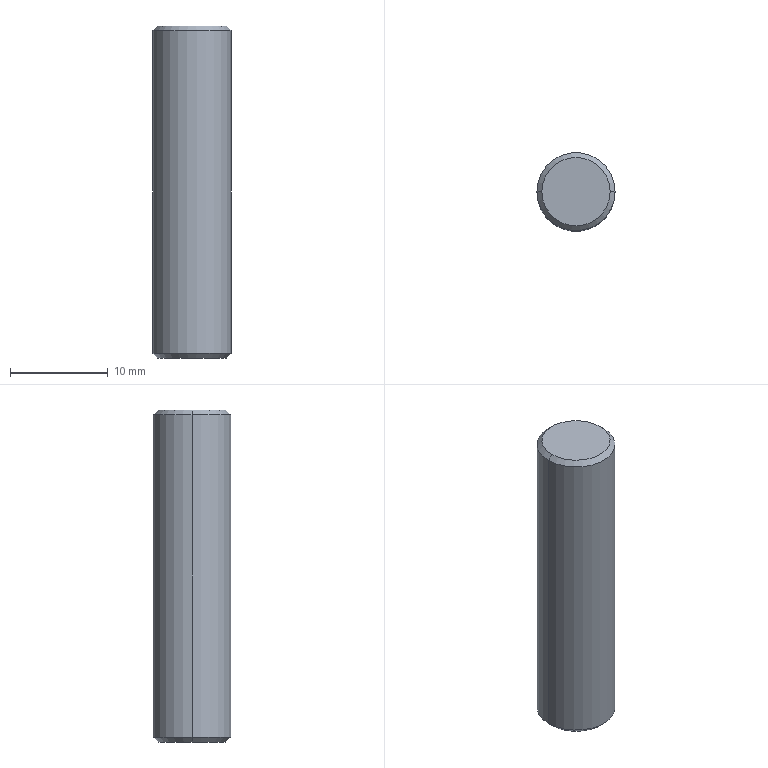Part | SolidWorks | features Chamfer 1, Extrusion 1 | 1 solid | 8 faces | box 8 x 8 x 34 mm | volume 1703 mm3 | cone 4 | cylinder 2 | plane 2 | commonest cylinder face diameters 8 x2
STEP:
#1=CARTESIAN_POINT('',(3.5,0.,17.));
#2=VERTEX_POINT('',#1);
#3=CARTESIAN_POINT('',(-3.5,0.,17.));
#4=VERTEX_POINT('',#3);
#5=CARTESIAN_POINT('',(0.,0.,17.));
#6=DIRECTION('',(0.,0.,1.));
#7=DIRECTION('',(1.,0.,0.));
#8=AXIS2_PLACEMENT_3D('',#5,#6,#7);
#9=CIRCLE('',#8,3.5);
#10=EDGE_CURVE('',#2,#4,#9,.T.);
#11=ORIENTED_EDGE('',*,*,#10,.F.);
#12=CARTESIAN_POINT('',(4.,0.,16.5));
#13=VERTEX_POINT('',#12);
#14=CARTESIAN_POINT('',(3.5,0.,17.));
#15=DIRECTION('',(0.7071,0.,-0.7071));
#16=VECTOR('',#15,1000.);
#17=LINE('',#14,#16);
#18=EDGE_CURVE('',#2,#13,#17,.T.);
#19=ORIENTED_EDGE('',*,*,#18,.T.);
#20=CARTESIAN_POINT('',(-4.,0.,16.5));
#21=VERTEX_POINT('',#20);
#22=CARTESIAN_POINT('',(0.,0.,16.5));
#23=DIRECTION('',(0.,0.,-1.));
#24=DIRECTION('',(1.,0.,0.));
#25=AXIS2_PLACEMENT_3D('',#22,#23,#24);
#26=CIRCLE('',#25,4.);
#27=EDGE_CURVE('',#21,#13,#26,.T.);
#28=ORIENTED_EDGE('',*,*,#27,.F.);
#29=CARTESIAN_POINT('',(-3.5,0.,17.));
#30=DIRECTION('',(-0.7071,0.,-0.7071));
#31=VECTOR('',#30,1000.);
#32=LINE('',#29,#31);
#33=EDGE_CURVE('',#4,#21,#32,.T.);
#34=ORIENTED_EDGE('',*,*,#33,.F.);
#35=EDGE_LOOP('',(#11,#19,#28,#34));
#36=FACE_OUTER_BOUND('',#35,.T.);
#37=CARTESIAN_POINT('',(0.,0.,17.));
#38=DIRECTION('',(0.,0.,-1.));
#39=DIRECTION('',(-1.,0.,0.));
#40=AXIS2_PLACEMENT_3D('',#37,#38,#39);
#41=CONICAL_SURFACE('',#40,3.5,0.7854);
#42=ADVANCED_FACE('',(#36),#41,.T.);
#43=CARTESIAN_POINT('',(-3.5,0.,-17.));
#44=VERTEX_POINT('',#43);
#45=CARTESIAN_POINT('',(3.5,0.,-17.));
#46=VERTEX_POINT('',#45);
#47=CARTESIAN_POINT('',(0.,0.,-17.));
#48=DIRECTION('',(0.,0.,-1.));
#49=DIRECTION('',(1.,0.,0.));
#50=AXIS2_PLACEMENT_3D('',#47,#48,#49);
#51=CIRCLE('',#50,3.5);
#52=EDGE_CURVE('',#44,#46,#51,.T.);
#53=ORIENTED_EDGE('',*,*,#52,.F.);
#54=CARTESIAN_POINT('',(-4.,0.,-16.5));
#55=VERTEX_POINT('',#54);
#56=CARTESIAN_POINT('',(-4.,0.,-16.5));
#57=DIRECTION('',(-0.7071,0.,0.7071));
#58=VECTOR('',#57,1000.);
#59=LINE('',#56,#58);
#60=EDGE_CURVE('',#44,#55,#59,.T.);
#61=ORIENTED_EDGE('',*,*,#60,.T.);
#62=CARTESIAN_POINT('',(4.,0.,-16.5));
#63=VERTEX_POINT('',#62);
#64=CARTESIAN_POINT('',(0.,0.,-16.5));
#65=DIRECTION('',(0.,0.,1.));
#66=DIRECTION('',(1.,0.,0.));
#67=AXIS2_PLACEMENT_3D('',#64,#65,#66);
#68=CIRCLE('',#67,4.);
#69=EDGE_CURVE('',#63,#55,#68,.T.);
#70=ORIENTED_EDGE('',*,*,#69,.F.);
#71=CARTESIAN_POINT('',(4.,0.,-16.5));
#72=DIRECTION('',(0.7071,0.,0.7071));
#73=VECTOR('',#72,1000.);
#74=LINE('',#71,#73);
#75=EDGE_CURVE('',#46,#63,#74,.T.);
#76=ORIENTED_EDGE('',*,*,#75,.F.);
#77=EDGE_LOOP('',(#53,#61,#70,#76));
#78=FACE_OUTER_BOUND('',#77,.T.);
#79=CARTESIAN_POINT('',(0.,0.,-16.5));
#80=DIRECTION('',(0.,0.,1.));
#81=DIRECTION('',(1.,0.,0.));
#82=AXIS2_PLACEMENT_3D('',#79,#80,#81);
#83=CONICAL_SURFACE('',#82,4.,0.7854);
#84=ADVANCED_FACE('',(#78),#83,.T.);
#85=ORIENTED_EDGE('',*,*,#27,.T.);
#86=CARTESIAN_POINT('',(4.,0.,17.));
#87=DIRECTION('',(0.,0.,-1.));
#88=VECTOR('',#87,1000.);
#89=LINE('',#86,#88);
#90=EDGE_CURVE('',#13,#63,#89,.T.);
#91=ORIENTED_EDGE('',*,*,#90,.T.);
#92=ORIENTED_EDGE('',*,*,#69,.T.);
#93=CARTESIAN_POINT('',(-4.,0.,17.));
#94=DIRECTION('',(0.,0.,-1.));
#95=VECTOR('',#94,1000.);
#96=LINE('',#93,#95);
#97=EDGE_CURVE('',#21,#55,#96,.T.);
#98=ORIENTED_EDGE('',*,*,#97,.F.);
#99=EDGE_LOOP('',(#85,#91,#92,#98));
#100=FACE_OUTER_BOUND('',#99,.T.);
#101=CARTESIAN_POINT('',(0.,0.,17.));
#102=DIRECTION('',(0.,0.,-1.));
#103=DIRECTION('',(-1.,0.,0.));
#104=AXIS2_PLACEMENT_3D('',#101,#102,#103);
#105=CYLINDRICAL_SURFACE('',#104,4.);
#106=ADVANCED_FACE('',(#100),#105,.T.);
#107=ORIENTED_EDGE('',*,*,#90,.F.);
#108=CARTESIAN_POINT('',(0.,0.,16.5));
#109=DIRECTION('',(0.,0.,-1.));
#110=DIRECTION('',(1.,0.,0.));
#111=AXIS2_PLACEMENT_3D('',#108,#109,#110);
#112=CIRCLE('',#111,4.);
#113=EDGE_CURVE('',#13,#21,#112,.T.);
#114=ORIENTED_EDGE('',*,*,#113,.T.);
#115=ORIENTED_EDGE('',*,*,#97,.T.);
#116=CARTESIAN_POINT('',(0.,0.,-16.5));
#117=DIRECTION('',(0.,0.,1.));
#118=DIRECTION('',(1.,0.,0.));
#119=AXIS2_PLACEMENT_3D('',#116,#117,#118);
#120=CIRCLE('',#119,4.);
#121=EDGE_CURVE('',#55,#63,#120,.T.);
#122=ORIENTED_EDGE('',*,*,#121,.T.);
#123=EDGE_LOOP('',(#107,#114,#115,#122));
#124=FACE_OUTER_BOUND('',#123,.T.);
#125=CARTESIAN_POINT('',(0.,0.,17.));
#126=DIRECTION('',(0.,0.,-1.));
#127=DIRECTION('',(-1.,0.,0.));
#128=AXIS2_PLACEMENT_3D('',#125,#126,#127);
#129=CYLINDRICAL_SURFACE('',#128,4.);
#130=ADVANCED_FACE('',(#124),#129,.T.);
#131=CARTESIAN_POINT('',(0.,0.,17.));
#132=DIRECTION('',(0.,0.,1.));
#133=DIRECTION('',(1.,0.,0.));
#134=AXIS2_PLACEMENT_3D('',#131,#132,#133);
#135=CIRCLE('',#134,3.5);
#136=EDGE_CURVE('',#4,#2,#135,.T.);
#137=ORIENTED_EDGE('',*,*,#136,.T.);
#138=ORIENTED_EDGE('',*,*,#10,.T.);
#139=EDGE_LOOP('',(#137,#138));
#140=FACE_OUTER_BOUND('',#139,.T.);
#141=CARTESIAN_POINT('',(0.,0.,17.));
#142=DIRECTION('',(0.,0.,1.));
#143=DIRECTION('',(1.,0.,0.));
#144=AXIS2_PLACEMENT_3D('',#141,#142,#143);
#145=PLANE('',#144);
#146=ADVANCED_FACE('',(#140),#145,.T.);
#147=CARTESIAN_POINT('',(0.,0.,-17.));
#148=DIRECTION('',(0.,0.,-1.));
#149=DIRECTION('',(1.,0.,0.));
#150=AXIS2_PLACEMENT_3D('',#147,#148,#149);
#151=CIRCLE('',#150,3.5);
#152=EDGE_CURVE('',#46,#44,#151,.T.);
#153=ORIENTED_EDGE('',*,*,#152,.T.);
#154=ORIENTED_EDGE('',*,*,#52,.T.);
#155=EDGE_LOOP('',(#153,#154));
#156=FACE_OUTER_BOUND('',#155,.T.);
#157=CARTESIAN_POINT('',(0.,0.,-17.));
#158=DIRECTION('',(0.,0.,1.));
#159=DIRECTION('',(1.,0.,0.));
#160=AXIS2_PLACEMENT_3D('',#157,#158,#159);
#161=PLANE('',#160);
#162=ADVANCED_FACE('',(#156),#161,.F.);
#163=ORIENTED_EDGE('',*,*,#60,.F.);
#164=ORIENTED_EDGE('',*,*,#152,.F.);
#165=ORIENTED_EDGE('',*,*,#75,.T.);
#166=ORIENTED_EDGE('',*,*,#121,.F.);
#167=EDGE_LOOP('',(#163,#164,#165,#166));
#168=FACE_OUTER_BOUND('',#167,.T.);
#169=CARTESIAN_POINT('',(0.,0.,-16.5));
#170=DIRECTION('',(0.,0.,1.));
#171=DIRECTION('',(1.,0.,0.));
#172=AXIS2_PLACEMENT_3D('',#169,#170,#171);
#173=CONICAL_SURFACE('',#172,4.,0.7854);
#174=ADVANCED_FACE('',(#168),#173,.T.);
#175=ORIENTED_EDGE('',*,*,#18,.F.);
#176=ORIENTED_EDGE('',*,*,#136,.F.);
#177=ORIENTED_EDGE('',*,*,#33,.T.);
#178=ORIENTED_EDGE('',*,*,#113,.F.);
#179=EDGE_LOOP('',(#175,#176,#177,#178));
#180=FACE_OUTER_BOUND('',#179,.T.);
#181=CARTESIAN_POINT('',(0.,0.,17.));
#182=DIRECTION('',(0.,0.,-1.));
#183=DIRECTION('',(-1.,0.,0.));
#184=AXIS2_PLACEMENT_3D('',#181,#182,#183);
#185=CONICAL_SURFACE('',#184,3.5,0.7854);
#186=ADVANCED_FACE('',(#180),#185,.T.);
#187=CLOSED_SHELL('',(#42,#84,#106,#130,#146,#162,#174,#186));
#188=MANIFOLD_SOLID_BREP('',#187);
#189=CARTESIAN_POINT('',(0.,0.,0.));
#190=DIRECTION('',(0.,0.,1.));
#191=DIRECTION('',(1.,0.,0.));
#192=AXIS2_PLACEMENT_3D('',#189,#190,#191);
#193=(LENGTH_UNIT()NAMED_UNIT(*)SI_UNIT(.MILLI.,.METRE.));
#194=UNCERTAINTY_MEASURE_WITH_UNIT(LENGTH_MEASURE(0.00001),#193,'','');
#195=(NAMED_UNIT(*)PLANE_ANGLE_UNIT()SI_UNIT($,.RADIAN.));
#196=(NAMED_UNIT(*)SI_UNIT($,.STERADIAN.)SOLID_ANGLE_UNIT());
#197=(GEOMETRIC_REPRESENTATION_CONTEXT(3)GLOBAL_UNCERTAINTY_ASSIGNED_CONTEXT((#194))GLOBAL_UNIT_ASSIGNED_CONTEXT((#193,#195,#196))REPRESENTATION_CONTEXT('',''));
#198=ADVANCED_BREP_SHAPE_REPRESENTATION('',(#188,#192),#197);